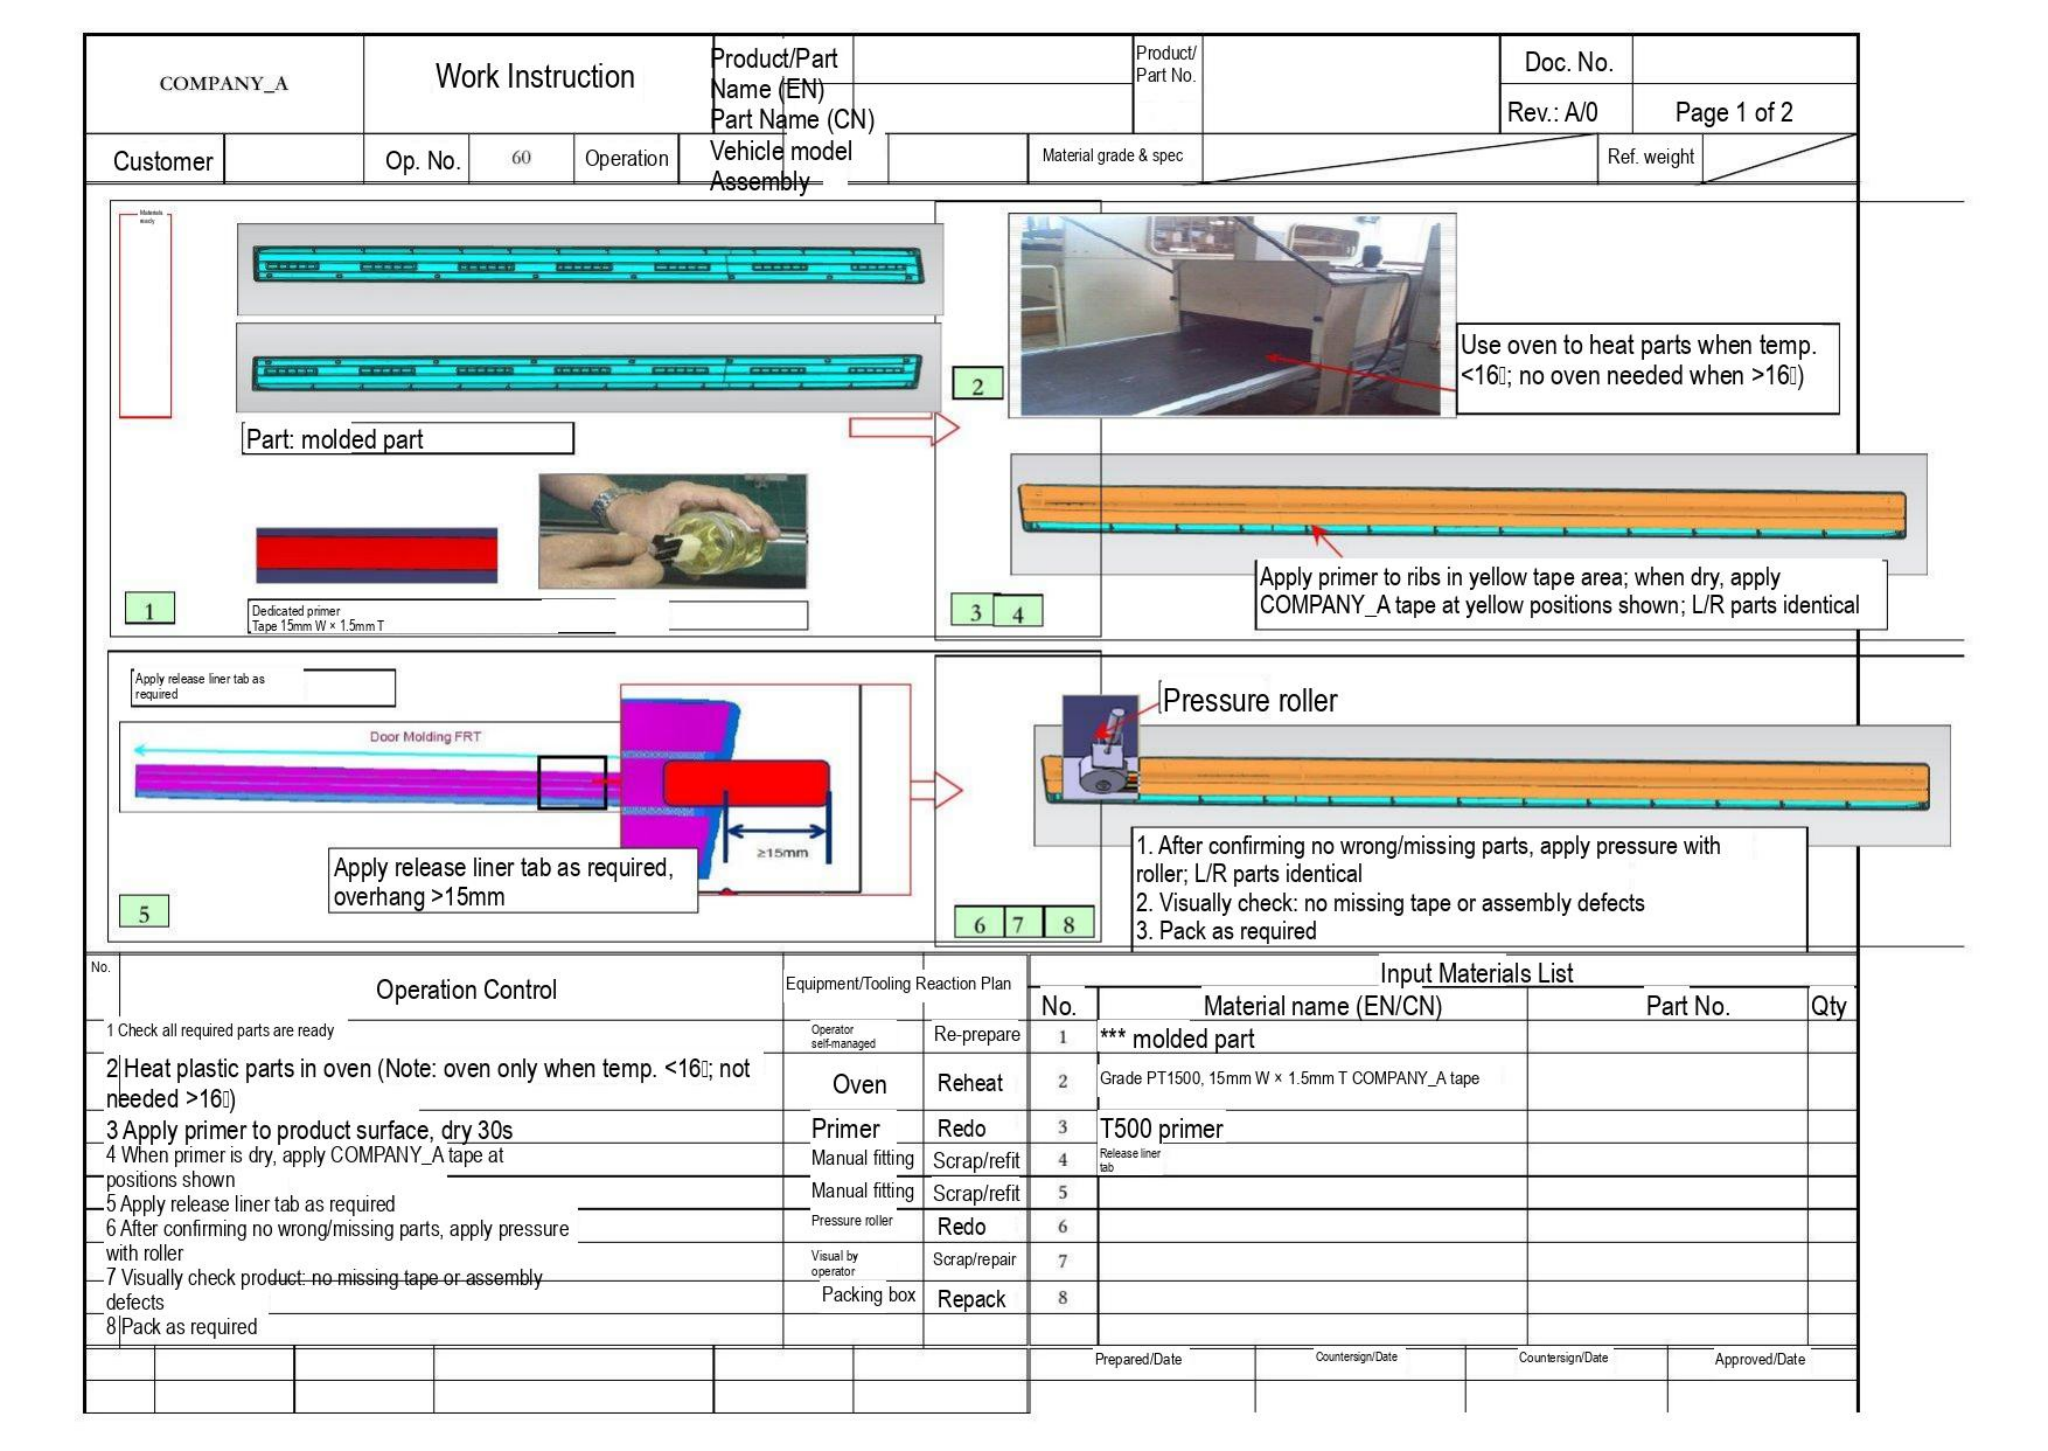**COMPANY_A** | **Work Instruction**

| | | | | | | | | | |
|---|---|---|---|---|---|---|---|---|---|
| COMPANY_A | Work Instruction | | Product/Part Name (EN) Part Name (CN) | | Product/ Part No. | | Doc. No. | | |
| | | | | | | | Rev.: A/0 | Page 1 of 2 | |
| Customer | | Op. No. | 60 | Operation | Vehicle model Assembly | | Material grade & spec | | Ref. weight |

Materials ready

Part: molded part

Dedicated primer
Tape 15mm W × 1.5mm T

1

2

Use oven to heat parts when temp. <16; no oven needed when >16)

3 4

Apply primer to ribs in yellow tape area; when dry, apply COMPANY_A tape at yellow positions shown; L/R parts identical

Apply release liner tab as required

Door Molding FRT

≥15mm

Apply release liner tab as required, overhang >15mm

5

Pressure roller

1. After confirming no wrong/missing parts, apply pressure with roller; L/R parts identical
2. Visually check: no missing tape or assembly defects
3. Pack as required

6 7 8

| No. | Operation Control | Equipment/Tooling | Reaction Plan |
|---|---|---|---|
| 1 | Check all required parts are ready | Operator self-managed | Re-prepare |
| 2 | Heat plastic parts in oven (Note: oven only when temp. <16; not needed >16) | Oven | Reheat |
| 3 | Apply primer to product surface, dry 30s | Primer | Redo |
| 4 | When primer is dry, apply COMPANY_A tape at positions shown | Manual fitting | Scrap/refit |
| 5 | Apply release liner tab as required | Manual fitting | Scrap/refit |
| 6 | After confirming no wrong/missing parts, apply pressure with roller | Pressure roller | Redo |
| 7 | Visually check product: no missing tape or assembly defects | Visual by operator | Scrap/repair |
| 8 | Pack as required | Packing box | Repack |

Input Materials List

| No. | Material name (EN/CN) | Part No. | Qty |
|---|---|---|---|
| 1 | *** molded part | | |
| 2 | Grade PT1500, 15mm W × 1.5mm T COMPANY_A tape | | |
| 3 | T500 primer | | |
| 4 | Release liner tab | | |
| 5 | | | |
| 6 | | | |
| 7 | | | |
| 8 | | | |

| Prepared/Date | Countersign/Date | Countersign/Date | Approved/Date |
|---|---|---|---|
| | | | |